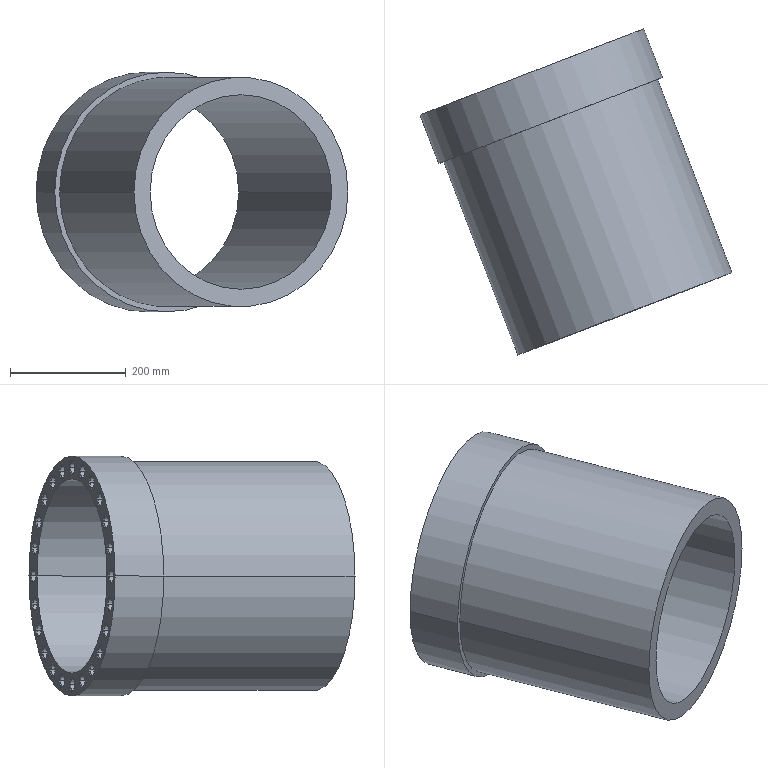Part | SolidWorks | features BaseBody 1, Scale 1 | 1 solid | 153 faces | box 538.702 x 563.166 x 414 mm | volume 15927299 mm3 | cone 96 | cylinder 54 | plane 3 | commonest cylinder face diameters 21 x48 336 x2 396 x2 414 x2